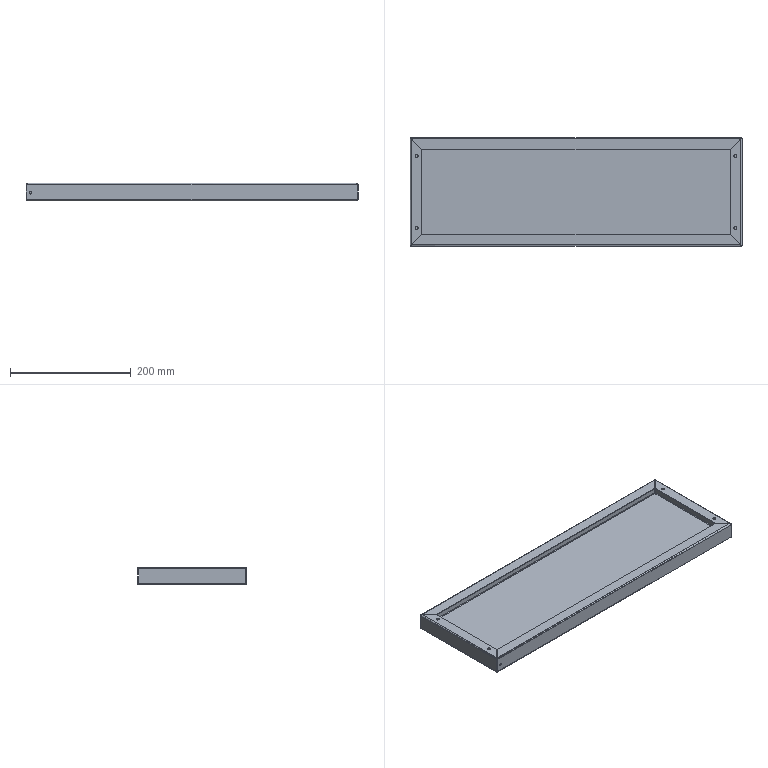Part | SolidWorks | features EdgeFlange 2, Cut 1, FlatPattern 1, ICE 1, SMBaseFlange 1, SheetMetal 1 | 1 solid | 80 faces | box 550 x 180 x 28.8 mm | volume 193683 mm3 | plane 38 | cylinder 26 | spline 16 | commonest cylinder face diameters 2 x8 4.4 x8 5 x8 4.2 x2